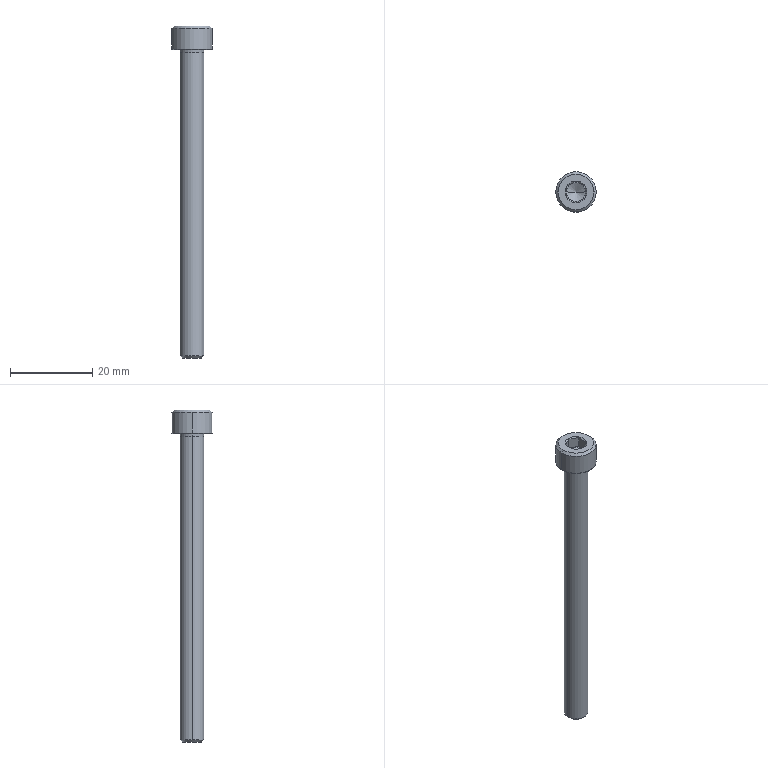Part | SolidWorks | features BaseBody 1 | 1 solid | 36 faces | box 9.808 x 9.808 x 80.769 mm | volume 2328 mm3 | cone 17 | plane 15 | cylinder 4 | commonest cylinder face diameters 5.769 x2 9.808 x2
STEP:
#1=CARTESIAN_POINT('',(233.792,130.07,193.643));
#2=VERTEX_POINT('',#1);
#3=CARTESIAN_POINT('',(228.023,130.07,193.643));
#4=VERTEX_POINT('',#3);
#5=CARTESIAN_POINT('',(230.907,130.07,193.643));
#6=DIRECTION('',(0.,0.,1.));
#7=DIRECTION('',(1.,0.,0.));
#8=AXIS2_PLACEMENT_3D('',#5,#6,#7);
#9=CIRCLE('',#8,2.885);
#10=EDGE_CURVE('',#2,#4,#9,.T.);
#11=ORIENTED_EDGE('',*,*,#10,.T.);
#12=CARTESIAN_POINT('',(228.023,130.07,267.385));
#13=VERTEX_POINT('',#12);
#14=CARTESIAN_POINT('',(228.023,130.07,193.077));
#15=DIRECTION('',(0.,0.,1.));
#16=VECTOR('',#15,1000.);
#17=LINE('',#14,#16);
#18=EDGE_CURVE('',#4,#13,#17,.T.);
#19=ORIENTED_EDGE('',*,*,#18,.T.);
#20=CARTESIAN_POINT('',(233.792,130.07,267.385));
#21=VERTEX_POINT('',#20);
#22=CARTESIAN_POINT('',(230.907,130.07,267.385));
#23=DIRECTION('',(0.,0.,-1.));
#24=DIRECTION('',(1.,0.,0.));
#25=AXIS2_PLACEMENT_3D('',#22,#23,#24);
#26=CIRCLE('',#25,2.885);
#27=EDGE_CURVE('',#13,#21,#26,.T.);
#28=ORIENTED_EDGE('',*,*,#27,.T.);
#29=CARTESIAN_POINT('',(233.792,130.07,193.077));
#30=DIRECTION('',(0.,0.,1.));
#31=VECTOR('',#30,1000.);
#32=LINE('',#29,#31);
#33=EDGE_CURVE('',#2,#21,#32,.T.);
#34=ORIENTED_EDGE('',*,*,#33,.F.);
#35=EDGE_LOOP('',(#11,#19,#28,#34));
#36=FACE_OUTER_BOUND('',#35,.T.);
#37=CARTESIAN_POINT('',(230.907,130.07,193.077));
#38=DIRECTION('',(0.,0.,1.));
#39=DIRECTION('',(1.,0.,0.));
#40=AXIS2_PLACEMENT_3D('',#37,#38,#39);
#41=CYLINDRICAL_SURFACE('',#40,2.885);
#42=ADVANCED_FACE('',(#36),#41,.T.);
#43=CARTESIAN_POINT('',(233.226,130.07,193.077));
#44=VERTEX_POINT('',#43);
#45=CARTESIAN_POINT('',(228.589,130.07,193.077));
#46=VERTEX_POINT('',#45);
#47=CARTESIAN_POINT('',(230.907,130.07,193.077));
#48=DIRECTION('',(0.,0.,1.));
#49=DIRECTION('',(1.,0.,0.));
#50=AXIS2_PLACEMENT_3D('',#47,#48,#49);
#51=CIRCLE('',#50,2.319);
#52=EDGE_CURVE('',#44,#46,#51,.T.);
#53=ORIENTED_EDGE('',*,*,#52,.T.);
#54=CARTESIAN_POINT('',(228.023,130.07,193.643));
#55=DIRECTION('',(-0.7071,0.,0.7071));
#56=VECTOR('',#55,1000.);
#57=LINE('',#54,#56);
#58=EDGE_CURVE('',#46,#4,#57,.T.);
#59=ORIENTED_EDGE('',*,*,#58,.T.);
#60=ORIENTED_EDGE('',*,*,#10,.F.);
#61=CARTESIAN_POINT('',(233.792,130.07,193.643));
#62=DIRECTION('',(0.7071,0.,0.7071));
#63=VECTOR('',#62,1000.);
#64=LINE('',#61,#63);
#65=EDGE_CURVE('',#44,#2,#64,.T.);
#66=ORIENTED_EDGE('',*,*,#65,.F.);
#67=EDGE_LOOP('',(#53,#59,#60,#66));
#68=FACE_OUTER_BOUND('',#67,.T.);
#69=CARTESIAN_POINT('',(230.907,130.07,193.643));
#70=DIRECTION('',(0.,0.,1.));
#71=DIRECTION('',(1.,0.,0.));
#72=AXIS2_PLACEMENT_3D('',#69,#70,#71);
#73=CONICAL_SURFACE('',#72,2.885,0.7854);
#74=ADVANCED_FACE('',(#68),#73,.T.);
#75=ORIENTED_EDGE('',*,*,#27,.F.);
#76=CARTESIAN_POINT('',(227.965,130.07,268.077));
#77=VERTEX_POINT('',#76);
#78=CARTESIAN_POINT('',(227.965,130.07,268.077));
#79=DIRECTION('',(-0.08305,0.,0.9965));
#80=VECTOR('',#79,1000.);
#81=LINE('',#78,#80);
#82=EDGE_CURVE('',#13,#77,#81,.T.);
#83=ORIENTED_EDGE('',*,*,#82,.T.);
#84=CARTESIAN_POINT('',(233.85,130.07,268.077));
#85=VERTEX_POINT('',#84);
#86=CARTESIAN_POINT('',(230.907,130.07,268.077));
#87=DIRECTION('',(0.,0.,-1.));
#88=DIRECTION('',(1.,0.,0.));
#89=AXIS2_PLACEMENT_3D('',#86,#87,#88);
#90=CIRCLE('',#89,2.942);
#91=EDGE_CURVE('',#77,#85,#90,.T.);
#92=ORIENTED_EDGE('',*,*,#91,.T.);
#93=CARTESIAN_POINT('',(233.85,130.07,268.077));
#94=DIRECTION('',(0.08305,0.,0.9965));
#95=VECTOR('',#94,1000.);
#96=LINE('',#93,#95);
#97=EDGE_CURVE('',#21,#85,#96,.T.);
#98=ORIENTED_EDGE('',*,*,#97,.F.);
#99=EDGE_LOOP('',(#75,#83,#92,#98));
#100=FACE_OUTER_BOUND('',#99,.T.);
#101=CARTESIAN_POINT('',(230.907,130.07,268.077));
#102=DIRECTION('',(0.,0.,1.));
#103=DIRECTION('',(1.,0.,0.));
#104=AXIS2_PLACEMENT_3D('',#101,#102,#103);
#105=CONICAL_SURFACE('',#104,2.942,0.08314);
#106=ADVANCED_FACE('',(#100),#105,.T.);
#107=CARTESIAN_POINT('',(235.667,130.07,268.077));
#108=VERTEX_POINT('',#107);
#109=CARTESIAN_POINT('',(226.148,130.07,268.077));
#110=VERTEX_POINT('',#109);
#111=CARTESIAN_POINT('',(230.907,130.07,268.077));
#112=DIRECTION('',(0.,0.,1.));
#113=DIRECTION('',(1.,0.,0.));
#114=AXIS2_PLACEMENT_3D('',#111,#112,#113);
#115=CIRCLE('',#114,4.76);
#116=EDGE_CURVE('',#108,#110,#115,.T.);
#117=ORIENTED_EDGE('',*,*,#116,.T.);
#118=CARTESIAN_POINT('',(226.004,130.07,268.221));
#119=VERTEX_POINT('',#118);
#120=CARTESIAN_POINT('',(226.004,130.07,268.221));
#121=DIRECTION('',(-0.7071,0.,0.7071));
#122=VECTOR('',#121,1000.);
#123=LINE('',#120,#122);
#124=EDGE_CURVE('',#110,#119,#123,.T.);
#125=ORIENTED_EDGE('',*,*,#124,.T.);
#126=CARTESIAN_POINT('',(235.811,130.07,268.221));
#127=VERTEX_POINT('',#126);
#128=CARTESIAN_POINT('',(230.907,130.07,268.221));
#129=DIRECTION('',(0.,0.,-1.));
#130=DIRECTION('',(0.,-1.,0.));
#131=AXIS2_PLACEMENT_3D('',#128,#129,#130);
#132=CIRCLE('',#131,4.904);
#133=EDGE_CURVE('',#119,#127,#132,.T.);
#134=ORIENTED_EDGE('',*,*,#133,.T.);
#135=CARTESIAN_POINT('',(235.811,130.07,268.221));
#136=DIRECTION('',(0.7071,0.,0.7071));
#137=VECTOR('',#136,1000.);
#138=LINE('',#135,#137);
#139=EDGE_CURVE('',#108,#127,#138,.T.);
#140=ORIENTED_EDGE('',*,*,#139,.F.);
#141=EDGE_LOOP('',(#117,#125,#134,#140));
#142=FACE_OUTER_BOUND('',#141,.T.);
#143=CARTESIAN_POINT('',(230.907,130.07,268.221));
#144=DIRECTION('',(0.,0.,1.));
#145=DIRECTION('',(1.,0.,0.));
#146=AXIS2_PLACEMENT_3D('',#143,#144,#145);
#147=CONICAL_SURFACE('',#146,4.904,0.7854);
#148=ADVANCED_FACE('',(#142),#147,.T.);
#149=ORIENTED_EDGE('',*,*,#133,.F.);
#150=CARTESIAN_POINT('',(226.004,130.07,273.269));
#151=VERTEX_POINT('',#150);
#152=CARTESIAN_POINT('',(226.004,130.07,193.077));
#153=DIRECTION('',(0.,0.,1.));
#154=VECTOR('',#153,1000.);
#155=LINE('',#152,#154);
#156=EDGE_CURVE('',#119,#151,#155,.T.);
#157=ORIENTED_EDGE('',*,*,#156,.T.);
#158=CARTESIAN_POINT('',(235.811,130.07,273.269));
#159=VERTEX_POINT('',#158);
#160=CARTESIAN_POINT('',(230.907,130.07,273.269));
#161=DIRECTION('',(0.,0.,-1.));
#162=DIRECTION('',(1.,0.,0.));
#163=AXIS2_PLACEMENT_3D('',#160,#161,#162);
#164=CIRCLE('',#163,4.904);
#165=EDGE_CURVE('',#151,#159,#164,.T.);
#166=ORIENTED_EDGE('',*,*,#165,.T.);
#167=CARTESIAN_POINT('',(235.811,130.07,193.077));
#168=DIRECTION('',(0.,0.,1.));
#169=VECTOR('',#168,1000.);
#170=LINE('',#167,#169);
#171=EDGE_CURVE('',#127,#159,#170,.T.);
#172=ORIENTED_EDGE('',*,*,#171,.F.);
#173=EDGE_LOOP('',(#149,#157,#166,#172));
#174=FACE_OUTER_BOUND('',#173,.T.);
#175=CARTESIAN_POINT('',(230.907,130.07,193.077));
#176=DIRECTION('',(0.,0.,1.));
#177=DIRECTION('',(1.,0.,0.));
#178=AXIS2_PLACEMENT_3D('',#175,#176,#177);
#179=CYLINDRICAL_SURFACE('',#178,4.904);
#180=ADVANCED_FACE('',(#174),#179,.T.);
#181=CARTESIAN_POINT('',(226.58,130.07,273.846));
#182=VERTEX_POINT('',#181);
#183=CARTESIAN_POINT('',(235.234,130.07,273.846));
#184=VERTEX_POINT('',#183);
#185=CARTESIAN_POINT('',(230.907,130.07,273.846));
#186=DIRECTION('',(0.,0.,-1.));
#187=DIRECTION('',(-1.,0.,0.));
#188=AXIS2_PLACEMENT_3D('',#185,#186,#187);
#189=CIRCLE('',#188,4.327);
#190=EDGE_CURVE('',#182,#184,#189,.T.);
#191=ORIENTED_EDGE('',*,*,#190,.T.);
#192=CARTESIAN_POINT('',(235.811,130.07,273.269));
#193=DIRECTION('',(0.7071,0.,-0.7071));
#194=VECTOR('',#193,1000.);
#195=LINE('',#192,#194);
#196=EDGE_CURVE('',#184,#159,#195,.T.);
#197=ORIENTED_EDGE('',*,*,#196,.T.);
#198=ORIENTED_EDGE('',*,*,#165,.F.);
#199=CARTESIAN_POINT('',(226.004,130.07,273.269));
#200=DIRECTION('',(-0.7071,0.,-0.7071));
#201=VECTOR('',#200,1000.);
#202=LINE('',#199,#201);
#203=EDGE_CURVE('',#182,#151,#202,.T.);
#204=ORIENTED_EDGE('',*,*,#203,.F.);
#205=EDGE_LOOP('',(#191,#197,#198,#204));
#206=FACE_OUTER_BOUND('',#205,.T.);
#207=CARTESIAN_POINT('',(230.907,130.07,273.269));
#208=DIRECTION('',(0.,0.,-1.));
#209=DIRECTION('',(-1.,0.,0.));
#210=AXIS2_PLACEMENT_3D('',#207,#208,#209);
#211=CONICAL_SURFACE('',#210,4.904,0.7854);
#212=ADVANCED_FACE('',(#206),#211,.T.);
#213=CARTESIAN_POINT('',(233.215,130.07,273.489));
#214=VERTEX_POINT('',#213);
#215=CARTESIAN_POINT('',(233.215,131.402,273.846));
#216=VERTEX_POINT('',#215);
#217=CARTESIAN_POINT('',(233.215,130.07,273.489));
#218=CARTESIAN_POINT('',(233.215,130.302,273.489));
#219=CARTESIAN_POINT('',(233.215,130.529,273.525));
#220=CARTESIAN_POINT('',(233.215,130.979,273.652));
#221=CARTESIAN_POINT('',(233.215,131.194,273.742));
#222=CARTESIAN_POINT('',(233.215,131.402,273.846));
#223=B_SPLINE_CURVE_WITH_KNOTS('',3,(#217,#218,#219,#220,#221,#222),.UNSPECIFIED.,.F.,.F.,(4,2,4),(0.001381,0.002067,0.002753),.UNSPECIFIED.);
#224=EDGE_CURVE('',#214,#216,#223,.T.);
#225=ORIENTED_EDGE('',*,*,#224,.F.);
#226=CARTESIAN_POINT('',(233.572,130.07,273.846));
#227=VERTEX_POINT('',#226);
#228=CARTESIAN_POINT('',(233.572,130.07,273.846));
#229=DIRECTION('',(0.7071,0.,0.7071));
#230=VECTOR('',#229,1000.);
#231=LINE('',#228,#230);
#232=EDGE_CURVE('',#214,#227,#231,.T.);
#233=ORIENTED_EDGE('',*,*,#232,.T.);
#234=CARTESIAN_POINT('',(230.907,130.07,273.846));
#235=DIRECTION('',(0.,0.,1.));
#236=DIRECTION('',(1.,0.,0.));
#237=AXIS2_PLACEMENT_3D('',#234,#235,#236);
#238=CIRCLE('',#237,2.665);
#239=EDGE_CURVE('',#227,#216,#238,.T.);
#240=ORIENTED_EDGE('',*,*,#239,.T.);
#241=EDGE_LOOP('',(#225,#233,#240));
#242=FACE_OUTER_BOUND('',#241,.T.);
#243=CARTESIAN_POINT('',(230.907,130.07,273.846));
#244=DIRECTION('',(0.,0.,1.));
#245=DIRECTION('',(1.,0.,0.));
#246=AXIS2_PLACEMENT_3D('',#243,#244,#245);
#247=CONICAL_SURFACE('',#246,2.665,0.7854);
#248=ADVANCED_FACE('',(#242),#247,.F.);
#249=CARTESIAN_POINT('',(230.907,130.07,269.629));
#250=VERTEX_POINT('',#249);
#251=CARTESIAN_POINT('',(233.215,130.07,270.962));
#252=VERTEX_POINT('',#251);
#253=CARTESIAN_POINT('',(233.215,130.07,270.962));
#254=DIRECTION('',(0.866,0.,0.5));
#255=VECTOR('',#254,1000.);
#256=LINE('',#253,#255);
#257=EDGE_CURVE('',#250,#252,#256,.T.);
#258=ORIENTED_EDGE('',*,*,#257,.F.);
#259=CARTESIAN_POINT('',(228.6,130.07,270.962));
#260=VERTEX_POINT('',#259);
#261=CARTESIAN_POINT('',(228.6,130.07,270.962));
#262=DIRECTION('',(-0.866,0.,0.5));
#263=VECTOR('',#262,1000.);
#264=LINE('',#261,#263);
#265=EDGE_CURVE('',#250,#260,#264,.T.);
#266=ORIENTED_EDGE('',*,*,#265,.T.);
#267=CARTESIAN_POINT('',(229.754,128.071,270.962));
#268=VERTEX_POINT('',#267);
#269=CARTESIAN_POINT('',(230.907,130.07,270.962));
#270=DIRECTION('',(0.,0.,-1.));
#271=DIRECTION('',(1.,0.,0.));
#272=AXIS2_PLACEMENT_3D('',#269,#270,#271);
#273=CIRCLE('',#272,2.308);
#274=EDGE_CURVE('',#268,#260,#273,.T.);
#275=ORIENTED_EDGE('',*,*,#274,.F.);
#276=CARTESIAN_POINT('',(232.061,128.071,270.962));
#277=VERTEX_POINT('',#276);
#278=CARTESIAN_POINT('',(230.907,130.07,270.962));
#279=DIRECTION('',(0.,0.,-1.));
#280=DIRECTION('',(1.,0.,0.));
#281=AXIS2_PLACEMENT_3D('',#278,#279,#280);
#282=CIRCLE('',#281,2.308);
#283=EDGE_CURVE('',#277,#268,#282,.T.);
#284=ORIENTED_EDGE('',*,*,#283,.F.);
#285=CARTESIAN_POINT('',(230.907,130.07,270.962));
#286=DIRECTION('',(0.,0.,-1.));
#287=DIRECTION('',(1.,0.,0.));
#288=AXIS2_PLACEMENT_3D('',#285,#286,#287);
#289=CIRCLE('',#288,2.308);
#290=EDGE_CURVE('',#252,#277,#289,.T.);
#291=ORIENTED_EDGE('',*,*,#290,.F.);
#292=EDGE_LOOP('',(#258,#266,#275,#284,#291));
#293=FACE_OUTER_BOUND('',#292,.T.);
#294=CARTESIAN_POINT('',(230.907,130.07,270.962));
#295=DIRECTION('',(0.,0.,1.));
#296=DIRECTION('',(1.,0.,0.));
#297=AXIS2_PLACEMENT_3D('',#294,#295,#296);
#298=CONICAL_SURFACE('',#297,2.308,1.047);
#299=ADVANCED_FACE('',(#293),#298,.F.);
#300=ORIENTED_EDGE('',*,*,#18,.F.);
#301=CARTESIAN_POINT('',(230.907,130.07,193.643));
#302=DIRECTION('',(0.,0.,1.));
#303=DIRECTION('',(1.,0.,0.));
#304=AXIS2_PLACEMENT_3D('',#301,#302,#303);
#305=CIRCLE('',#304,2.885);
#306=EDGE_CURVE('',#4,#2,#305,.T.);
#307=ORIENTED_EDGE('',*,*,#306,.T.);
#308=ORIENTED_EDGE('',*,*,#33,.T.);
#309=CARTESIAN_POINT('',(230.907,130.07,267.385));
#310=DIRECTION('',(0.,0.,-1.));
#311=DIRECTION('',(1.,0.,0.));
#312=AXIS2_PLACEMENT_3D('',#309,#310,#311);
#313=CIRCLE('',#312,2.885);
#314=EDGE_CURVE('',#21,#13,#313,.T.);
#315=ORIENTED_EDGE('',*,*,#314,.T.);
#316=EDGE_LOOP('',(#300,#307,#308,#315));
#317=FACE_OUTER_BOUND('',#316,.T.);
#318=CARTESIAN_POINT('',(230.907,130.07,193.077));
#319=DIRECTION('',(0.,0.,1.));
#320=DIRECTION('',(1.,0.,0.));
#321=AXIS2_PLACEMENT_3D('',#318,#319,#320);
#322=CYLINDRICAL_SURFACE('',#321,2.885);
#323=ADVANCED_FACE('',(#317),#322,.T.);
#324=ORIENTED_EDGE('',*,*,#58,.F.);
#325=CARTESIAN_POINT('',(230.907,130.07,193.077));
#326=DIRECTION('',(0.,0.,1.));
#327=DIRECTION('',(1.,0.,0.));
#328=AXIS2_PLACEMENT_3D('',#325,#326,#327);
#329=CIRCLE('',#328,2.319);
#330=EDGE_CURVE('',#46,#44,#329,.T.);
#331=ORIENTED_EDGE('',*,*,#330,.T.);
#332=ORIENTED_EDGE('',*,*,#65,.T.);
#333=ORIENTED_EDGE('',*,*,#306,.F.);
#334=EDGE_LOOP('',(#324,#331,#332,#333));
#335=FACE_OUTER_BOUND('',#334,.T.);
#336=CARTESIAN_POINT('',(230.907,130.07,193.643));
#337=DIRECTION('',(0.,0.,1.));
#338=DIRECTION('',(1.,0.,0.));
#339=AXIS2_PLACEMENT_3D('',#336,#337,#338);
#340=CONICAL_SURFACE('',#339,2.885,0.7854);
#341=ADVANCED_FACE('',(#335),#340,.T.);
#342=ORIENTED_EDGE('',*,*,#82,.F.);
#343=ORIENTED_EDGE('',*,*,#314,.F.);
#344=ORIENTED_EDGE('',*,*,#97,.T.);
#345=CARTESIAN_POINT('',(230.907,130.07,268.077));
#346=DIRECTION('',(0.,0.,-1.));
#347=DIRECTION('',(1.,0.,0.));
#348=AXIS2_PLACEMENT_3D('',#345,#346,#347);
#349=CIRCLE('',#348,2.942);
#350=EDGE_CURVE('',#85,#77,#349,.T.);
#351=ORIENTED_EDGE('',*,*,#350,.T.);
#352=EDGE_LOOP('',(#342,#343,#344,#351));
#353=FACE_OUTER_BOUND('',#352,.T.);
#354=CARTESIAN_POINT('',(230.907,130.07,268.077));
#355=DIRECTION('',(0.,0.,1.));
#356=DIRECTION('',(1.,0.,0.));
#357=AXIS2_PLACEMENT_3D('',#354,#355,#356);
#358=CONICAL_SURFACE('',#357,2.942,0.08314);
#359=ADVANCED_FACE('',(#353),#358,.T.);
#360=ORIENTED_EDGE('',*,*,#52,.F.);
#361=ORIENTED_EDGE('',*,*,#330,.F.);
#362=EDGE_LOOP('',(#360,#361));
#363=FACE_OUTER_BOUND('',#362,.T.);
#364=CARTESIAN_POINT('',(228.589,130.07,193.077));
#365=DIRECTION('',(0.,0.,1.));
#366=DIRECTION('',(1.,0.,0.));
#367=AXIS2_PLACEMENT_3D('',#364,#365,#366);
#368=PLANE('',#367);
#369=ADVANCED_FACE('',(#363),#368,.F.);
#370=ORIENTED_EDGE('',*,*,#350,.F.);
#371=ORIENTED_EDGE('',*,*,#91,.F.);
#372=EDGE_LOOP('',(#370,#371));
#373=FACE_BOUND('',#372,.T.);
#374=ORIENTED_EDGE('',*,*,#116,.F.);
#375=CARTESIAN_POINT('',(230.907,130.07,268.077));
#376=DIRECTION('',(0.,0.,1.));
#377=DIRECTION('',(1.,0.,0.));
#378=AXIS2_PLACEMENT_3D('',#375,#376,#377);
#379=CIRCLE('',#378,4.76);
#380=EDGE_CURVE('',#110,#108,#379,.T.);
#381=ORIENTED_EDGE('',*,*,#380,.F.);
#382=EDGE_LOOP('',(#374,#381));
#383=FACE_OUTER_BOUND('',#382,.T.);
#384=CARTESIAN_POINT('',(226.148,130.07,268.077));
#385=DIRECTION('',(0.,0.,1.));
#386=DIRECTION('',(1.,0.,0.));
#387=AXIS2_PLACEMENT_3D('',#384,#385,#386);
#388=PLANE('',#387);
#389=ADVANCED_FACE('',(#373,#383),#388,.F.);
#390=ORIENTED_EDGE('',*,*,#124,.F.);
#391=ORIENTED_EDGE('',*,*,#380,.T.);
#392=ORIENTED_EDGE('',*,*,#139,.T.);
#393=CARTESIAN_POINT('',(230.907,130.07,268.221));
#394=DIRECTION('',(0.,0.,-1.));
#395=DIRECTION('',(0.,-1.,0.));
#396=AXIS2_PLACEMENT_3D('',#393,#394,#395);
#397=CIRCLE('',#396,4.904);
#398=EDGE_CURVE('',#127,#119,#397,.T.);
#399=ORIENTED_EDGE('',*,*,#398,.T.);
#400=EDGE_LOOP('',(#390,#391,#392,#399));
#401=FACE_OUTER_BOUND('',#400,.T.);
#402=CARTESIAN_POINT('',(230.907,130.07,268.221));
#403=DIRECTION('',(0.,0.,1.));
#404=DIRECTION('',(1.,0.,0.));
#405=AXIS2_PLACEMENT_3D('',#402,#403,#404);
#406=CONICAL_SURFACE('',#405,4.904,0.7854);
#407=ADVANCED_FACE('',(#401),#406,.T.);
#408=ORIENTED_EDGE('',*,*,#156,.F.);
#409=ORIENTED_EDGE('',*,*,#398,.F.);
#410=ORIENTED_EDGE('',*,*,#171,.T.);
#411=CARTESIAN_POINT('',(230.907,130.07,273.269));
#412=DIRECTION('',(0.,0.,-1.));
#413=DIRECTION('',(1.,0.,0.));
#414=AXIS2_PLACEMENT_3D('',#411,#412,#413);
#415=CIRCLE('',#414,4.904);
#416=EDGE_CURVE('',#159,#151,#415,.T.);
#417=ORIENTED_EDGE('',*,*,#416,.T.);
#418=EDGE_LOOP('',(#408,#409,#410,#417));
#419=FACE_OUTER_BOUND('',#418,.T.);
#420=CARTESIAN_POINT('',(230.907,130.07,193.077));
#421=DIRECTION('',(0.,0.,1.));
#422=DIRECTION('',(1.,0.,0.));
#423=AXIS2_PLACEMENT_3D('',#420,#421,#422);
#424=CYLINDRICAL_SURFACE('',#423,4.904);
#425=ADVANCED_FACE('',(#419),#424,.T.);
#426=ORIENTED_EDGE('',*,*,#196,.F.);
#427=CARTESIAN_POINT('',(230.907,130.07,273.846));
#428=DIRECTION('',(0.,0.,-1.));
#429=DIRECTION('',(-1.,0.,0.));
#430=AXIS2_PLACEMENT_3D('',#427,#428,#429);
#431=CIRCLE('',#430,4.327);
#432=EDGE_CURVE('',#184,#182,#431,.T.);
#433=ORIENTED_EDGE('',*,*,#432,.T.);
#434=ORIENTED_EDGE('',*,*,#203,.T.);
#435=ORIENTED_EDGE('',*,*,#416,.F.);
#436=EDGE_LOOP('',(#426,#433,#434,#435));
#437=FACE_OUTER_BOUND('',#436,.T.);
#438=CARTESIAN_POINT('',(230.907,130.07,273.269));
#439=DIRECTION('',(0.,0.,-1.));
#440=DIRECTION('',(-1.,0.,0.));
#441=AXIS2_PLACEMENT_3D('',#438,#439,#440);
#442=CONICAL_SURFACE('',#441,4.904,0.7854);
#443=ADVANCED_FACE('',(#437),#442,.T.);
#444=CARTESIAN_POINT('',(230.907,132.735,273.846));
#445=VERTEX_POINT('',#444);
#446=CARTESIAN_POINT('',(230.907,130.07,273.846));
#447=DIRECTION('',(0.,0.,1.));
#448=DIRECTION('',(1.,0.,0.));
#449=AXIS2_PLACEMENT_3D('',#446,#447,#448);
#450=CIRCLE('',#449,2.665);
#451=EDGE_CURVE('',#216,#445,#450,.T.);
#452=ORIENTED_EDGE('',*,*,#451,.F.);
#453=ORIENTED_EDGE('',*,*,#239,.F.);
#454=CARTESIAN_POINT('',(233.215,128.738,273.846));
#455=VERTEX_POINT('',#454);
#456=CARTESIAN_POINT('',(230.907,130.07,273.846));
#457=DIRECTION('',(0.,0.,1.));
#458=DIRECTION('',(1.,0.,0.));
#459=AXIS2_PLACEMENT_3D('',#456,#457,#458);
#460=CIRCLE('',#459,2.665);
#461=EDGE_CURVE('',#455,#227,#460,.T.);
#462=ORIENTED_EDGE('',*,*,#461,.F.);
#463=CARTESIAN_POINT('',(230.907,127.405,273.846));
#464=VERTEX_POINT('',#463);
#465=CARTESIAN_POINT('',(230.907,130.07,273.846));
#466=DIRECTION('',(0.,0.,1.));
#467=DIRECTION('',(1.,0.,0.));
#468=AXIS2_PLACEMENT_3D('',#465,#466,#467);
#469=CIRCLE('',#468,2.665);
#470=EDGE_CURVE('',#464,#455,#469,.T.);
#471=ORIENTED_EDGE('',*,*,#470,.F.);
#472=CARTESIAN_POINT('',(228.6,128.738,273.846));
#473=VERTEX_POINT('',#472);
#474=CARTESIAN_POINT('',(230.907,130.07,273.846));
#475=DIRECTION('',(0.,0.,1.));
#476=DIRECTION('',(1.,0.,0.));
#477=AXIS2_PLACEMENT_3D('',#474,#475,#476);
#478=CIRCLE('',#477,2.665);
#479=EDGE_CURVE('',#473,#464,#478,.T.);
#480=ORIENTED_EDGE('',*,*,#479,.F.);
#481=CARTESIAN_POINT('',(228.6,131.402,273.846));
#482=VERTEX_POINT('',#481);
#483=CARTESIAN_POINT('',(230.907,130.07,273.846));
#484=DIRECTION('',(0.,0.,1.));
#485=DIRECTION('',(1.,0.,0.));
#486=AXIS2_PLACEMENT_3D('',#483,#484,#485);
#487=CIRCLE('',#486,2.665);
#488=EDGE_CURVE('',#482,#473,#487,.T.);
#489=ORIENTED_EDGE('',*,*,#488,.F.);
#490=CARTESIAN_POINT('',(230.907,130.07,273.846));
#491=DIRECTION('',(0.,0.,1.));
#492=DIRECTION('',(1.,0.,0.));
#493=AXIS2_PLACEMENT_3D('',#490,#491,#492);
#494=CIRCLE('',#493,2.665);
#495=EDGE_CURVE('',#445,#482,#494,.T.);
#496=ORIENTED_EDGE('',*,*,#495,.F.);
#497=EDGE_LOOP('',(#452,#453,#462,#471,#480,#489,#496));
#498=FACE_BOUND('',#497,.T.);
#499=ORIENTED_EDGE('',*,*,#190,.F.);
#500=ORIENTED_EDGE('',*,*,#432,.F.);
#501=EDGE_LOOP('',(#499,#500));
#502=FACE_OUTER_BOUND('',#501,.T.);
#503=CARTESIAN_POINT('',(228.243,130.07,273.846));
#504=DIRECTION('',(0.,0.,-1.));
#505=DIRECTION('',(-1.,0.,0.));
#506=AXIS2_PLACEMENT_3D('',#503,#504,#505);
#507=PLANE('',#506);
#508=ADVANCED_FACE('',(#498,#502),#507,.F.);
#509=CARTESIAN_POINT('',(230.907,132.735,273.846));
#510=CARTESIAN_POINT('',(230.727,132.631,273.742));
#511=CARTESIAN_POINT('',(230.543,132.524,273.654));
#512=CARTESIAN_POINT('',(230.256,132.359,273.559));
#513=CARTESIAN_POINT('',(230.159,132.303,273.533));
#514=CARTESIAN_POINT('',(229.961,132.188,273.499));
#515=CARTESIAN_POINT('',(229.859,132.129,273.489));
#516=CARTESIAN_POINT('',(229.556,131.955,273.489));
#517=CARTESIAN_POINT('',(229.358,131.84,273.524));
#518=CARTESIAN_POINT('',(228.968,131.615,273.652));
#519=CARTESIAN_POINT('',(228.781,131.507,273.741));
#520=CARTESIAN_POINT('',(228.6,131.402,273.846));
#521=B_SPLINE_CURVE_WITH_KNOTS('',3,(#509,#510,#511,#512,#513,#514,#515,#516,#517,#518,#519,#520),.UNSPECIFIED.,.F.,.F.,(4,2,2,2,2,4),(0.,0.0006881,0.001032,0.001376,0.002064,0.002753),.UNSPECIFIED.);
#522=EDGE_CURVE('',#445,#482,#521,.T.);
#523=ORIENTED_EDGE('',*,*,#522,.F.);
#524=ORIENTED_EDGE('',*,*,#495,.T.);
#525=EDGE_LOOP('',(#523,#524));
#526=FACE_OUTER_BOUND('',#525,.T.);
#527=CARTESIAN_POINT('',(230.907,130.07,273.846));
#528=DIRECTION('',(0.,0.,1.));
#529=DIRECTION('',(1.,0.,0.));
#530=AXIS2_PLACEMENT_3D('',#527,#528,#529);
#531=CONICAL_SURFACE('',#530,2.665,0.7854);
#532=ADVANCED_FACE('',(#526),#531,.F.);
#533=CARTESIAN_POINT('',(233.215,131.402,273.846));
#534=CARTESIAN_POINT('',(233.035,131.506,273.742));
#535=CARTESIAN_POINT('',(232.85,131.613,273.654));
#536=CARTESIAN_POINT('',(232.564,131.778,273.559));
#537=CARTESIAN_POINT('',(232.467,131.834,273.533));
#538=CARTESIAN_POINT('',(232.268,131.949,273.499));
#539=CARTESIAN_POINT('',(232.166,132.008,273.489));
#540=CARTESIAN_POINT('',(231.864,132.182,273.489));
#541=CARTESIAN_POINT('',(231.666,132.297,273.524));
#542=CARTESIAN_POINT('',(231.276,132.522,273.652));
#543=CARTESIAN_POINT('',(231.089,132.63,273.741));
#544=CARTESIAN_POINT('',(230.907,132.735,273.846));
#545=B_SPLINE_CURVE_WITH_KNOTS('',3,(#533,#534,#535,#536,#537,#538,#539,#540,#541,#542,#543,#544),.UNSPECIFIED.,.F.,.F.,(4,2,2,2,2,4),(0.,0.0006881,0.001032,0.001376,0.002064,0.002753),.UNSPECIFIED.);
#546=EDGE_CURVE('',#216,#445,#545,.T.);
#547=ORIENTED_EDGE('',*,*,#546,.F.);
#548=ORIENTED_EDGE('',*,*,#451,.T.);
#549=EDGE_LOOP('',(#547,#548));
#550=FACE_OUTER_BOUND('',#549,.T.);
#551=CARTESIAN_POINT('',(230.907,130.07,273.846));
#552=DIRECTION('',(0.,0.,1.));
#553=DIRECTION('',(1.,0.,0.));
#554=AXIS2_PLACEMENT_3D('',#551,#552,#553);
#555=CONICAL_SURFACE('',#554,2.665,0.7854);
#556=ADVANCED_FACE('',(#550),#555,.F.);
#557=ORIENTED_EDGE('',*,*,#232,.F.);
#558=CARTESIAN_POINT('',(233.215,128.738,273.846));
#559=CARTESIAN_POINT('',(233.215,128.947,273.742));
#560=CARTESIAN_POINT('',(233.215,129.16,273.653));
#561=CARTESIAN_POINT('',(233.215,129.492,273.558));
#562=CARTESIAN_POINT('',(233.215,129.605,273.533));
#563=CARTESIAN_POINT('',(233.215,129.835,273.498));
#564=CARTESIAN_POINT('',(233.215,129.953,273.489));
#565=CARTESIAN_POINT('',(233.215,130.07,273.489));
#566=B_SPLINE_CURVE_WITH_KNOTS('',3,(#558,#559,#560,#561,#562,#563,#564,#565),.UNSPECIFIED.,.F.,.F.,(4,2,2,4),(0.,0.0006905,0.001036,0.001381),.UNSPECIFIED.);
#567=EDGE_CURVE('',#455,#214,#566,.T.);
#568=ORIENTED_EDGE('',*,*,#567,.F.);
#569=ORIENTED_EDGE('',*,*,#461,.T.);
#570=EDGE_LOOP('',(#557,#568,#569));
#571=FACE_OUTER_BOUND('',#570,.T.);
#572=CARTESIAN_POINT('',(230.907,130.07,273.846));
#573=DIRECTION('',(0.,0.,1.));
#574=DIRECTION('',(1.,0.,0.));
#575=AXIS2_PLACEMENT_3D('',#572,#573,#574);
#576=CONICAL_SURFACE('',#575,2.665,0.7854);
#577=ADVANCED_FACE('',(#571),#576,.F.);
#578=CARTESIAN_POINT('',(230.907,127.405,273.846));
#579=CARTESIAN_POINT('',(231.088,127.509,273.742));
#580=CARTESIAN_POINT('',(231.272,127.616,273.654));
#581=CARTESIAN_POINT('',(231.559,127.781,273.559));
#582=CARTESIAN_POINT('',(231.656,127.837,273.533));
#583=CARTESIAN_POINT('',(231.854,127.952,273.499));
#584=CARTESIAN_POINT('',(231.956,128.011,273.489));
#585=CARTESIAN_POINT('',(232.258,128.185,273.489));
#586=CARTESIAN_POINT('',(232.456,128.3,273.524));
#587=CARTESIAN_POINT('',(232.847,128.525,273.652));
#588=CARTESIAN_POINT('',(233.034,128.633,273.741));
#589=CARTESIAN_POINT('',(233.215,128.738,273.846));
#590=B_SPLINE_CURVE_WITH_KNOTS('',3,(#578,#579,#580,#581,#582,#583,#584,#585,#586,#587,#588,#589),.UNSPECIFIED.,.F.,.F.,(4,2,2,2,2,4),(0.,0.0006881,0.001032,0.001376,0.002064,0.002753),.UNSPECIFIED.);
#591=EDGE_CURVE('',#464,#455,#590,.T.);
#592=ORIENTED_EDGE('',*,*,#591,.F.);
#593=ORIENTED_EDGE('',*,*,#470,.T.);
#594=EDGE_LOOP('',(#592,#593));
#595=FACE_OUTER_BOUND('',#594,.T.);
#596=CARTESIAN_POINT('',(230.907,130.07,273.846));
#597=DIRECTION('',(0.,0.,1.));
#598=DIRECTION('',(1.,0.,0.));
#599=AXIS2_PLACEMENT_3D('',#596,#597,#598);
#600=CONICAL_SURFACE('',#599,2.665,0.7854);
#601=ADVANCED_FACE('',(#595),#600,.F.);
#602=CARTESIAN_POINT('',(228.6,128.738,273.846));
#603=CARTESIAN_POINT('',(228.78,128.633,273.742));
#604=CARTESIAN_POINT('',(228.964,128.527,273.654));
#605=CARTESIAN_POINT('',(229.251,128.362,273.559));
#606=CARTESIAN_POINT('',(229.348,128.306,273.533));
#607=CARTESIAN_POINT('',(229.546,128.191,273.499));
#608=CARTESIAN_POINT('',(229.649,128.132,273.489));
#609=CARTESIAN_POINT('',(229.951,127.958,273.489));
#610=CARTESIAN_POINT('',(230.149,127.843,273.524));
#611=CARTESIAN_POINT('',(230.539,127.618,273.652));
#612=CARTESIAN_POINT('',(230.726,127.51,273.741));
#613=CARTESIAN_POINT('',(230.907,127.405,273.846));
#614=B_SPLINE_CURVE_WITH_KNOTS('',3,(#602,#603,#604,#605,#606,#607,#608,#609,#610,#611,#612,#613),.UNSPECIFIED.,.F.,.F.,(4,2,2,2,2,4),(0.,0.0006881,0.001032,0.001376,0.002064,0.002753),.UNSPECIFIED.);
#615=EDGE_CURVE('',#473,#464,#614,.T.);
#616=ORIENTED_EDGE('',*,*,#615,.F.);
#617=ORIENTED_EDGE('',*,*,#479,.T.);
#618=EDGE_LOOP('',(#616,#617));
#619=FACE_OUTER_BOUND('',#618,.T.);
#620=CARTESIAN_POINT('',(230.907,130.07,273.846));
#621=DIRECTION('',(0.,0.,1.));
#622=DIRECTION('',(1.,0.,0.));
#623=AXIS2_PLACEMENT_3D('',#620,#621,#622);
#624=CONICAL_SURFACE('',#623,2.665,0.7854);
#625=ADVANCED_FACE('',(#619),#624,.F.);
#626=CARTESIAN_POINT('',(228.6,131.402,273.846));
#627=CARTESIAN_POINT('',(228.6,131.194,273.742));
#628=CARTESIAN_POINT('',(228.6,130.981,273.654));
#629=CARTESIAN_POINT('',(228.6,130.65,273.559));
#630=CARTESIAN_POINT('',(228.6,130.538,273.533));
#631=CARTESIAN_POINT('',(228.6,130.309,273.499));
#632=CARTESIAN_POINT('',(228.6,130.191,273.489));
#633=CARTESIAN_POINT('',(228.6,129.842,273.489));
#634=CARTESIAN_POINT('',(228.6,129.614,273.524));
#635=CARTESIAN_POINT('',(228.6,129.163,273.652));
#636=CARTESIAN_POINT('',(228.6,128.947,273.741));
#637=CARTESIAN_POINT('',(228.6,128.738,273.846));
#638=B_SPLINE_CURVE_WITH_KNOTS('',3,(#626,#627,#628,#629,#630,#631,#632,#633,#634,#635,#636,#637),.UNSPECIFIED.,.F.,.F.,(4,2,2,2,2,4),(0.,0.0006881,0.001032,0.001376,0.002064,0.002753),.UNSPECIFIED.);
#639=EDGE_CURVE('',#482,#473,#638,.T.);
#640=ORIENTED_EDGE('',*,*,#639,.F.);
#641=ORIENTED_EDGE('',*,*,#488,.T.);
#642=EDGE_LOOP('',(#640,#641));
#643=FACE_OUTER_BOUND('',#642,.T.);
#644=CARTESIAN_POINT('',(230.907,130.07,273.846));
#645=DIRECTION('',(0.,0.,1.));
#646=DIRECTION('',(1.,0.,0.));
#647=AXIS2_PLACEMENT_3D('',#644,#645,#646);
#648=CONICAL_SURFACE('',#647,2.665,0.7854);
#649=ADVANCED_FACE('',(#643),#648,.F.);
#650=CARTESIAN_POINT('',(228.6,131.402,270.962));
#651=VERTEX_POINT('',#650);
#652=CARTESIAN_POINT('',(228.6,131.402,270.962));
#653=DIRECTION('',(0.,0.,1.));
#654=VECTOR('',#653,1000.);
#655=LINE('',#652,#654);
#656=EDGE_CURVE('',#651,#482,#655,.T.);
#657=ORIENTED_EDGE('',*,*,#656,.F.);
#658=CARTESIAN_POINT('',(229.754,132.068,270.962));
#659=VERTEX_POINT('',#658);
#660=CARTESIAN_POINT('',(230.907,132.735,270.962));
#661=DIRECTION('',(-0.866,-0.5,0.));
#662=VECTOR('',#661,1000.);
#663=LINE('',#660,#662);
#664=EDGE_CURVE('',#659,#651,#663,.T.);
#665=ORIENTED_EDGE('',*,*,#664,.F.);
#666=CARTESIAN_POINT('',(230.907,132.735,270.962));
#667=VERTEX_POINT('',#666);
#668=CARTESIAN_POINT('',(230.907,132.735,270.962));
#669=DIRECTION('',(-0.866,-0.5,0.));
#670=VECTOR('',#669,1000.);
#671=LINE('',#668,#670);
#672=EDGE_CURVE('',#667,#659,#671,.T.);
#673=ORIENTED_EDGE('',*,*,#672,.F.);
#674=CARTESIAN_POINT('',(230.907,132.735,270.962));
#675=DIRECTION('',(0.,0.,-1.));
#676=VECTOR('',#675,1000.);
#677=LINE('',#674,#676);
#678=EDGE_CURVE('',#445,#667,#677,.T.);
#679=ORIENTED_EDGE('',*,*,#678,.F.);
#680=ORIENTED_EDGE('',*,*,#522,.T.);
#681=EDGE_LOOP('',(#657,#665,#673,#679,#680));
#682=FACE_OUTER_BOUND('',#681,.T.);
#683=CARTESIAN_POINT('',(230.907,132.735,270.962));
#684=DIRECTION('',(-0.5,0.866,0.));
#685=DIRECTION('',(-0.866,-0.5,0.));
#686=AXIS2_PLACEMENT_3D('',#683,#684,#685);
#687=PLANE('',#686);
#688=ADVANCED_FACE('',(#682),#687,.F.);
#689=ORIENTED_EDGE('',*,*,#678,.T.);
#690=CARTESIAN_POINT('',(232.061,132.068,270.962));
#691=VERTEX_POINT('',#690);
#692=CARTESIAN_POINT('',(233.215,131.402,270.962));
#693=DIRECTION('',(-0.866,0.5,0.));
#694=VECTOR('',#693,1000.);
#695=LINE('',#692,#694);
#696=EDGE_CURVE('',#691,#667,#695,.T.);
#697=ORIENTED_EDGE('',*,*,#696,.F.);
#698=CARTESIAN_POINT('',(233.215,131.402,270.962));
#699=VERTEX_POINT('',#698);
#700=CARTESIAN_POINT('',(233.215,131.402,270.962));
#701=DIRECTION('',(-0.866,0.5,0.));
#702=VECTOR('',#701,1000.);
#703=LINE('',#700,#702);
#704=EDGE_CURVE('',#699,#691,#703,.T.);
#705=ORIENTED_EDGE('',*,*,#704,.F.);
#706=CARTESIAN_POINT('',(233.215,131.402,270.962));
#707=DIRECTION('',(0.,0.,-1.));
#708=VECTOR('',#707,1000.);
#709=LINE('',#706,#708);
#710=EDGE_CURVE('',#216,#699,#709,.T.);
#711=ORIENTED_EDGE('',*,*,#710,.F.);
#712=ORIENTED_EDGE('',*,*,#546,.T.);
#713=EDGE_LOOP('',(#689,#697,#705,#711,#712));
#714=FACE_OUTER_BOUND('',#713,.T.);
#715=CARTESIAN_POINT('',(233.215,131.402,270.962));
#716=DIRECTION('',(0.5,0.866,0.));
#717=DIRECTION('',(-0.866,0.5,0.));
#718=AXIS2_PLACEMENT_3D('',#715,#716,#717);
#719=PLANE('',#718);
#720=ADVANCED_FACE('',(#714),#719,.F.);
#721=ORIENTED_EDGE('',*,*,#710,.T.);
#722=CARTESIAN_POINT('',(233.215,128.738,270.962));
#723=DIRECTION('',(0.,1.,0.));
#724=VECTOR('',#723,1000.);
#725=LINE('',#722,#724);
#726=EDGE_CURVE('',#252,#699,#725,.T.);
#727=ORIENTED_EDGE('',*,*,#726,.F.);
#728=CARTESIAN_POINT('',(233.215,128.738,270.962));
#729=VERTEX_POINT('',#728);
#730=CARTESIAN_POINT('',(233.215,128.738,270.962));
#731=DIRECTION('',(0.,1.,0.));
#732=VECTOR('',#731,1000.);
#733=LINE('',#730,#732);
#734=EDGE_CURVE('',#729,#252,#733,.T.);
#735=ORIENTED_EDGE('',*,*,#734,.F.);
#736=CARTESIAN_POINT('',(233.215,128.738,270.962));
#737=DIRECTION('',(0.,0.,-1.));
#738=VECTOR('',#737,1000.);
#739=LINE('',#736,#738);
#740=EDGE_CURVE('',#455,#729,#739,.T.);
#741=ORIENTED_EDGE('',*,*,#740,.F.);
#742=ORIENTED_EDGE('',*,*,#567,.T.);
#743=ORIENTED_EDGE('',*,*,#224,.T.);
#744=EDGE_LOOP('',(#721,#727,#735,#741,#742,#743));
#745=FACE_OUTER_BOUND('',#744,.T.);
#746=CARTESIAN_POINT('',(233.215,128.738,270.962));
#747=DIRECTION('',(1.,0.,0.));
#748=DIRECTION('',(0.,0.,-1.));
#749=AXIS2_PLACEMENT_3D('',#746,#747,#748);
#750=PLANE('',#749);
#751=ADVANCED_FACE('',(#745),#750,.F.);
#752=ORIENTED_EDGE('',*,*,#740,.T.);
#753=CARTESIAN_POINT('',(230.907,127.405,270.962));
#754=DIRECTION('',(0.866,0.5,0.));
#755=VECTOR('',#754,1000.);
#756=LINE('',#753,#755);
#757=EDGE_CURVE('',#277,#729,#756,.T.);
#758=ORIENTED_EDGE('',*,*,#757,.F.);
#759=CARTESIAN_POINT('',(230.907,127.405,270.962));
#760=VERTEX_POINT('',#759);
#761=CARTESIAN_POINT('',(230.907,127.405,270.962));
#762=DIRECTION('',(0.866,0.5,0.));
#763=VECTOR('',#762,1000.);
#764=LINE('',#761,#763);
#765=EDGE_CURVE('',#760,#277,#764,.T.);
#766=ORIENTED_EDGE('',*,*,#765,.F.);
#767=CARTESIAN_POINT('',(230.907,127.405,270.962));
#768=DIRECTION('',(0.,0.,-1.));
#769=VECTOR('',#768,1000.);
#770=LINE('',#767,#769);
#771=EDGE_CURVE('',#464,#760,#770,.T.);
#772=ORIENTED_EDGE('',*,*,#771,.F.);
#773=ORIENTED_EDGE('',*,*,#591,.T.);
#774=EDGE_LOOP('',(#752,#758,#766,#772,#773));
#775=FACE_OUTER_BOUND('',#774,.T.);
#776=CARTESIAN_POINT('',(230.907,127.405,270.962));
#777=DIRECTION('',(0.5,-0.866,0.));
#778=DIRECTION('',(0.866,0.5,0.));
#779=AXIS2_PLACEMENT_3D('',#776,#777,#778);
#780=PLANE('',#779);
#781=ADVANCED_FACE('',(#775),#780,.F.);
#782=ORIENTED_EDGE('',*,*,#771,.T.);
#783=CARTESIAN_POINT('',(228.6,128.738,270.962));
#784=DIRECTION('',(0.866,-0.5,0.));
#785=VECTOR('',#784,1000.);
#786=LINE('',#783,#785);
#787=EDGE_CURVE('',#268,#760,#786,.T.);
#788=ORIENTED_EDGE('',*,*,#787,.F.);
#789=CARTESIAN_POINT('',(228.6,128.738,270.962));
#790=VERTEX_POINT('',#789);
#791=CARTESIAN_POINT('',(228.6,128.738,270.962));
#792=DIRECTION('',(0.866,-0.5,0.));
#793=VECTOR('',#792,1000.);
#794=LINE('',#791,#793);
#795=EDGE_CURVE('',#790,#268,#794,.T.);
#796=ORIENTED_EDGE('',*,*,#795,.F.);
#797=CARTESIAN_POINT('',(228.6,128.738,270.962));
#798=DIRECTION('',(0.,0.,-1.));
#799=VECTOR('',#798,1000.);
#800=LINE('',#797,#799);
#801=EDGE_CURVE('',#473,#790,#800,.T.);
#802=ORIENTED_EDGE('',*,*,#801,.F.);
#803=ORIENTED_EDGE('',*,*,#615,.T.);
#804=EDGE_LOOP('',(#782,#788,#796,#802,#803));
#805=FACE_OUTER_BOUND('',#804,.T.);
#806=CARTESIAN_POINT('',(228.6,128.738,270.962));
#807=DIRECTION('',(-0.5,-0.866,0.));
#808=DIRECTION('',(0.866,-0.5,0.));
#809=AXIS2_PLACEMENT_3D('',#806,#807,#808);
#810=PLANE('',#809);
#811=ADVANCED_FACE('',(#805),#810,.F.);
#812=ORIENTED_EDGE('',*,*,#801,.T.);
#813=CARTESIAN_POINT('',(228.6,131.402,270.962));
#814=DIRECTION('',(0.,-1.,0.));
#815=VECTOR('',#814,1000.);
#816=LINE('',#813,#815);
#817=EDGE_CURVE('',#260,#790,#816,.T.);
#818=ORIENTED_EDGE('',*,*,#817,.F.);
#819=CARTESIAN_POINT('',(228.6,131.402,270.962));
#820=DIRECTION('',(0.,-1.,0.));
#821=VECTOR('',#820,1000.);
#822=LINE('',#819,#821);
#823=EDGE_CURVE('',#651,#260,#822,.T.);
#824=ORIENTED_EDGE('',*,*,#823,.F.);
#825=ORIENTED_EDGE('',*,*,#656,.T.);
#826=ORIENTED_EDGE('',*,*,#639,.T.);
#827=EDGE_LOOP('',(#812,#818,#824,#825,#826));
#828=FACE_OUTER_BOUND('',#827,.T.);
#829=CARTESIAN_POINT('',(228.6,131.402,270.962));
#830=DIRECTION('',(-1.,0.,0.));
#831=DIRECTION('',(0.,0.,1.));
#832=AXIS2_PLACEMENT_3D('',#829,#830,#831);
#833=PLANE('',#832);
#834=ADVANCED_FACE('',(#828),#833,.F.);
#835=CARTESIAN_POINT('',(230.907,130.07,270.962));
#836=DIRECTION('',(0.,0.,-1.));
#837=DIRECTION('',(1.,0.,0.));
#838=AXIS2_PLACEMENT_3D('',#835,#836,#837);
#839=CIRCLE('',#838,2.308);
#840=EDGE_CURVE('',#260,#659,#839,.T.);
#841=ORIENTED_EDGE('',*,*,#840,.T.);
#842=ORIENTED_EDGE('',*,*,#664,.T.);
#843=ORIENTED_EDGE('',*,*,#823,.T.);
#844=EDGE_LOOP('',(#841,#842,#843));
#845=FACE_OUTER_BOUND('',#844,.T.);
#846=CARTESIAN_POINT('',(230.907,130.07,270.962));
#847=DIRECTION('',(0.,0.,1.));
#848=DIRECTION('',(1.,0.,0.));
#849=AXIS2_PLACEMENT_3D('',#846,#847,#848);
#850=PLANE('',#849);
#851=ADVANCED_FACE('',(#845),#850,.T.);
#852=CARTESIAN_POINT('',(230.907,130.07,270.962));
#853=DIRECTION('',(0.,0.,-1.));
#854=DIRECTION('',(1.,0.,0.));
#855=AXIS2_PLACEMENT_3D('',#852,#853,#854);
#856=CIRCLE('',#855,2.308);
#857=EDGE_CURVE('',#659,#691,#856,.T.);
#858=ORIENTED_EDGE('',*,*,#857,.T.);
#859=ORIENTED_EDGE('',*,*,#696,.T.);
#860=ORIENTED_EDGE('',*,*,#672,.T.);
#861=EDGE_LOOP('',(#858,#859,#860));
#862=FACE_OUTER_BOUND('',#861,.T.);
#863=CARTESIAN_POINT('',(230.907,130.07,270.962));
#864=DIRECTION('',(0.,0.,1.));
#865=DIRECTION('',(1.,0.,0.));
#866=AXIS2_PLACEMENT_3D('',#863,#864,#865);
#867=PLANE('',#866);
#868=ADVANCED_FACE('',(#862),#867,.T.);
#869=CARTESIAN_POINT('',(230.907,130.07,270.962));
#870=DIRECTION('',(0.,0.,-1.));
#871=DIRECTION('',(1.,0.,0.));
#872=AXIS2_PLACEMENT_3D('',#869,#870,#871);
#873=CIRCLE('',#872,2.308);
#874=EDGE_CURVE('',#691,#252,#873,.T.);
#875=ORIENTED_EDGE('',*,*,#874,.T.);
#876=ORIENTED_EDGE('',*,*,#726,.T.);
#877=ORIENTED_EDGE('',*,*,#704,.T.);
#878=EDGE_LOOP('',(#875,#876,#877));
#879=FACE_OUTER_BOUND('',#878,.T.);
#880=CARTESIAN_POINT('',(230.907,130.07,270.962));
#881=DIRECTION('',(0.,0.,1.));
#882=DIRECTION('',(1.,0.,0.));
#883=AXIS2_PLACEMENT_3D('',#880,#881,#882);
#884=PLANE('',#883);
#885=ADVANCED_FACE('',(#879),#884,.T.);
#886=ORIENTED_EDGE('',*,*,#290,.T.);
#887=ORIENTED_EDGE('',*,*,#757,.T.);
#888=ORIENTED_EDGE('',*,*,#734,.T.);
#889=EDGE_LOOP('',(#886,#887,#888));
#890=FACE_OUTER_BOUND('',#889,.T.);
#891=CARTESIAN_POINT('',(230.907,130.07,270.962));
#892=DIRECTION('',(0.,0.,1.));
#893=DIRECTION('',(1.,0.,0.));
#894=AXIS2_PLACEMENT_3D('',#891,#892,#893);
#895=PLANE('',#894);
#896=ADVANCED_FACE('',(#890),#895,.T.);
#897=ORIENTED_EDGE('',*,*,#283,.T.);
#898=ORIENTED_EDGE('',*,*,#787,.T.);
#899=ORIENTED_EDGE('',*,*,#765,.T.);
#900=EDGE_LOOP('',(#897,#898,#899));
#901=FACE_OUTER_BOUND('',#900,.T.);
#902=CARTESIAN_POINT('',(230.907,130.07,270.962));
#903=DIRECTION('',(0.,0.,1.));
#904=DIRECTION('',(1.,0.,0.));
#905=AXIS2_PLACEMENT_3D('',#902,#903,#904);
#906=PLANE('',#905);
#907=ADVANCED_FACE('',(#901),#906,.T.);
#908=ORIENTED_EDGE('',*,*,#274,.T.);
#909=ORIENTED_EDGE('',*,*,#817,.T.);
#910=ORIENTED_EDGE('',*,*,#795,.T.);
#911=EDGE_LOOP('',(#908,#909,#910));
#912=FACE_OUTER_BOUND('',#911,.T.);
#913=CARTESIAN_POINT('',(230.907,130.07,270.962));
#914=DIRECTION('',(0.,0.,1.));
#915=DIRECTION('',(1.,0.,0.));
#916=AXIS2_PLACEMENT_3D('',#913,#914,#915);
#917=PLANE('',#916);
#918=ADVANCED_FACE('',(#912),#917,.T.);
#919=ORIENTED_EDGE('',*,*,#265,.F.);
#920=ORIENTED_EDGE('',*,*,#257,.T.);
#921=ORIENTED_EDGE('',*,*,#874,.F.);
#922=ORIENTED_EDGE('',*,*,#857,.F.);
#923=ORIENTED_EDGE('',*,*,#840,.F.);
#924=EDGE_LOOP('',(#919,#920,#921,#922,#923));
#925=FACE_OUTER_BOUND('',#924,.T.);
#926=CARTESIAN_POINT('',(230.907,130.07,270.962));
#927=DIRECTION('',(0.,0.,1.));
#928=DIRECTION('',(1.,0.,0.));
#929=AXIS2_PLACEMENT_3D('',#926,#927,#928);
#930=CONICAL_SURFACE('',#929,2.308,1.047);
#931=ADVANCED_FACE('',(#925),#930,.F.);
#932=CLOSED_SHELL('',(#42,#74,#106,#148,#180,#212,#248,#299,#323,#341,#359,#369,#389,#407,#425,#443,#508,#532,#556,#577,#601,#625,#649,#688,#720,#751,#781,#811,#834,#851,#868,#885,#896,#907,#918,#931));
#933=MANIFOLD_SOLID_BREP('',#932);
#934=CARTESIAN_POINT('',(0.,0.,0.));
#935=DIRECTION('',(0.,0.,1.));
#936=DIRECTION('',(1.,0.,0.));
#937=AXIS2_PLACEMENT_3D('',#934,#935,#936);
#938=(LENGTH_UNIT()NAMED_UNIT(*)SI_UNIT(.MILLI.,.METRE.));
#939=UNCERTAINTY_MEASURE_WITH_UNIT(LENGTH_MEASURE(0.00001),#938,'','');
#940=(NAMED_UNIT(*)PLANE_ANGLE_UNIT()SI_UNIT($,.RADIAN.));
#941=(NAMED_UNIT(*)SI_UNIT($,.STERADIAN.)SOLID_ANGLE_UNIT());
#942=(GEOMETRIC_REPRESENTATION_CONTEXT(3)GLOBAL_UNCERTAINTY_ASSIGNED_CONTEXT((#939))GLOBAL_UNIT_ASSIGNED_CONTEXT((#938,#940,#941))REPRESENTATION_CONTEXT('',''));
#943=ADVANCED_BREP_SHAPE_REPRESENTATION('',(#933,#937),#942);